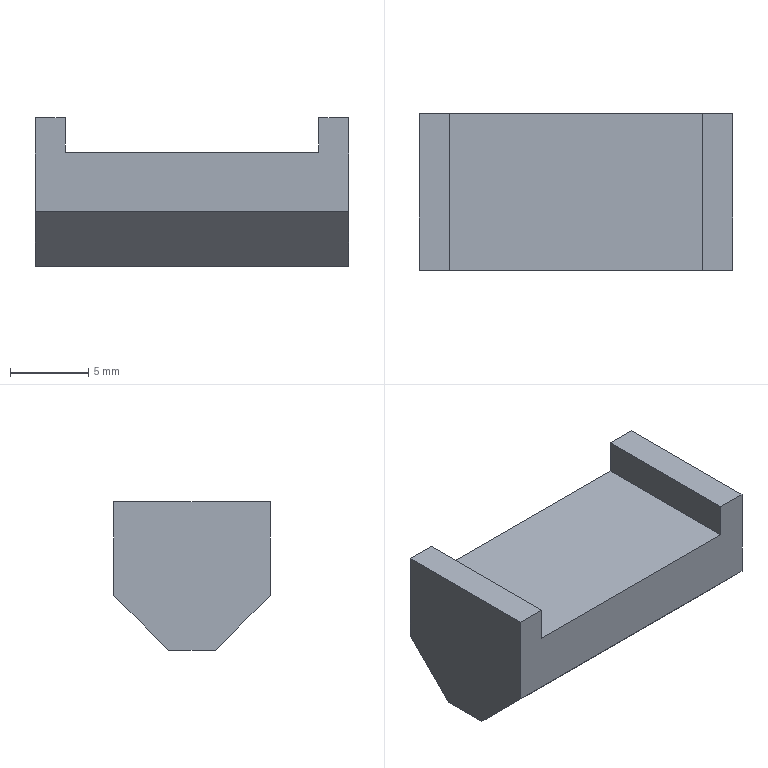Part | SolidWorks | features ICE 2, Extrusion 1, MirrorPattern 1 | 1 solid | 12 faces | box 20 x 10 x 9.5 mm | volume 1299 mm3 | plane 12
STEP:
#1=CARTESIAN_POINT('',(-10.,-1.5,0.));
#2=VERTEX_POINT('',#1);
#3=CARTESIAN_POINT('',(-10.,-5.,3.5));
#4=VERTEX_POINT('',#3);
#5=CARTESIAN_POINT('',(-10.,-5.,3.5));
#6=DIRECTION('',(0.,-0.7071,0.7071));
#7=VECTOR('',#6,1000.);
#8=LINE('',#5,#7);
#9=EDGE_CURVE('',#2,#4,#8,.T.);
#10=ORIENTED_EDGE('',*,*,#9,.T.);
#11=CARTESIAN_POINT('',(-10.,-5.,9.5));
#12=VERTEX_POINT('',#11);
#13=CARTESIAN_POINT('',(-10.,-5.,9.5));
#14=DIRECTION('',(0.,0.,-1.));
#15=VECTOR('',#14,1000.);
#16=LINE('',#13,#15);
#17=EDGE_CURVE('',#12,#4,#16,.T.);
#18=ORIENTED_EDGE('',*,*,#17,.F.);
#19=CARTESIAN_POINT('',(-10.,5.,9.5));
#20=VERTEX_POINT('',#19);
#21=CARTESIAN_POINT('',(-10.,5.,9.5));
#22=DIRECTION('',(0.,-1.,0.));
#23=VECTOR('',#22,1000.);
#24=LINE('',#21,#23);
#25=EDGE_CURVE('',#20,#12,#24,.T.);
#26=ORIENTED_EDGE('',*,*,#25,.F.);
#27=CARTESIAN_POINT('',(-10.,5.,3.5));
#28=VERTEX_POINT('',#27);
#29=CARTESIAN_POINT('',(-10.,5.,9.5));
#30=DIRECTION('',(0.,0.,-1.));
#31=VECTOR('',#30,1000.);
#32=LINE('',#29,#31);
#33=EDGE_CURVE('',#20,#28,#32,.T.);
#34=ORIENTED_EDGE('',*,*,#33,.T.);
#35=CARTESIAN_POINT('',(-10.,1.5,0.));
#36=VERTEX_POINT('',#35);
#37=CARTESIAN_POINT('',(-10.,5.,3.5));
#38=DIRECTION('',(0.,0.7071,0.7071));
#39=VECTOR('',#38,1000.);
#40=LINE('',#37,#39);
#41=EDGE_CURVE('',#36,#28,#40,.T.);
#42=ORIENTED_EDGE('',*,*,#41,.F.);
#43=CARTESIAN_POINT('',(-10.,5.,0.));
#44=DIRECTION('',(0.,-1.,0.));
#45=VECTOR('',#44,1000.);
#46=LINE('',#43,#45);
#47=EDGE_CURVE('',#36,#2,#46,.T.);
#48=ORIENTED_EDGE('',*,*,#47,.T.);
#49=EDGE_LOOP('',(#10,#18,#26,#34,#42,#48));
#50=FACE_OUTER_BOUND('',#49,.T.);
#51=CARTESIAN_POINT('',(-10.,5.,9.5));
#52=DIRECTION('',(1.,0.,0.));
#53=DIRECTION('',(0.,0.,-1.));
#54=AXIS2_PLACEMENT_3D('',#51,#52,#53);
#55=PLANE('',#54);
#56=ADVANCED_FACE('',(#50),#55,.F.);
#57=CARTESIAN_POINT('',(10.,-5.,3.5));
#58=VERTEX_POINT('',#57);
#59=CARTESIAN_POINT('',(10.,-5.,3.5));
#60=DIRECTION('',(-1.,0.,0.));
#61=VECTOR('',#60,1000.);
#62=LINE('',#59,#61);
#63=EDGE_CURVE('',#58,#4,#62,.T.);
#64=ORIENTED_EDGE('',*,*,#63,.F.);
#65=CARTESIAN_POINT('',(10.,-5.,9.5));
#66=VERTEX_POINT('',#65);
#67=CARTESIAN_POINT('',(10.,-5.,9.5));
#68=DIRECTION('',(0.,0.,-1.));
#69=VECTOR('',#68,1000.);
#70=LINE('',#67,#69);
#71=EDGE_CURVE('',#66,#58,#70,.T.);
#72=ORIENTED_EDGE('',*,*,#71,.F.);
#73=CARTESIAN_POINT('',(8.1,-5.,9.5));
#74=VERTEX_POINT('',#73);
#75=CARTESIAN_POINT('',(-10.,-5.,9.5));
#76=DIRECTION('',(1.,0.,0.));
#77=VECTOR('',#76,1000.);
#78=LINE('',#75,#77);
#79=EDGE_CURVE('',#74,#66,#78,.T.);
#80=ORIENTED_EDGE('',*,*,#79,.F.);
#81=CARTESIAN_POINT('',(8.1,-5.,7.3));
#82=VERTEX_POINT('',#81);
#83=CARTESIAN_POINT('',(8.1,-5.,9.5));
#84=DIRECTION('',(0.,0.,-1.));
#85=VECTOR('',#84,1000.);
#86=LINE('',#83,#85);
#87=EDGE_CURVE('',#74,#82,#86,.T.);
#88=ORIENTED_EDGE('',*,*,#87,.T.);
#89=CARTESIAN_POINT('',(-8.1,-5.,7.3));
#90=VERTEX_POINT('',#89);
#91=CARTESIAN_POINT('',(-10.,-5.,7.3));
#92=DIRECTION('',(1.,0.,0.));
#93=VECTOR('',#92,1000.);
#94=LINE('',#91,#93);
#95=EDGE_CURVE('',#90,#82,#94,.T.);
#96=ORIENTED_EDGE('',*,*,#95,.F.);
#97=CARTESIAN_POINT('',(-8.1,-5.,9.5));
#98=VERTEX_POINT('',#97);
#99=CARTESIAN_POINT('',(-8.1,-5.,9.5));
#100=DIRECTION('',(0.,0.,1.));
#101=VECTOR('',#100,1000.);
#102=LINE('',#99,#101);
#103=EDGE_CURVE('',#90,#98,#102,.T.);
#104=ORIENTED_EDGE('',*,*,#103,.T.);
#105=CARTESIAN_POINT('',(-10.,-5.,9.5));
#106=DIRECTION('',(1.,0.,0.));
#107=VECTOR('',#106,1000.);
#108=LINE('',#105,#107);
#109=EDGE_CURVE('',#12,#98,#108,.T.);
#110=ORIENTED_EDGE('',*,*,#109,.F.);
#111=ORIENTED_EDGE('',*,*,#17,.T.);
#112=EDGE_LOOP('',(#64,#72,#80,#88,#96,#104,#110,#111));
#113=FACE_OUTER_BOUND('',#112,.T.);
#114=CARTESIAN_POINT('',(-10.,-5.,9.5));
#115=DIRECTION('',(0.,1.,0.));
#116=DIRECTION('',(0.,0.,1.));
#117=AXIS2_PLACEMENT_3D('',#114,#115,#116);
#118=PLANE('',#117);
#119=ADVANCED_FACE('',(#113),#118,.F.);
#120=CARTESIAN_POINT('',(10.,-1.5,0.));
#121=VERTEX_POINT('',#120);
#122=CARTESIAN_POINT('',(10.,-5.,3.5));
#123=DIRECTION('',(0.,-0.7071,0.7071));
#124=VECTOR('',#123,1000.);
#125=LINE('',#122,#124);
#126=EDGE_CURVE('',#121,#58,#125,.T.);
#127=ORIENTED_EDGE('',*,*,#126,.F.);
#128=CARTESIAN_POINT('',(10.,1.5,0.));
#129=VERTEX_POINT('',#128);
#130=CARTESIAN_POINT('',(10.,5.,0.));
#131=DIRECTION('',(0.,1.,0.));
#132=VECTOR('',#131,1000.);
#133=LINE('',#130,#132);
#134=EDGE_CURVE('',#121,#129,#133,.T.);
#135=ORIENTED_EDGE('',*,*,#134,.T.);
#136=CARTESIAN_POINT('',(10.,5.,3.5));
#137=VERTEX_POINT('',#136);
#138=CARTESIAN_POINT('',(10.,5.,3.5));
#139=DIRECTION('',(0.,0.7071,0.7071));
#140=VECTOR('',#139,1000.);
#141=LINE('',#138,#140);
#142=EDGE_CURVE('',#129,#137,#141,.T.);
#143=ORIENTED_EDGE('',*,*,#142,.T.);
#144=CARTESIAN_POINT('',(10.,5.,9.5));
#145=VERTEX_POINT('',#144);
#146=CARTESIAN_POINT('',(10.,5.,9.5));
#147=DIRECTION('',(0.,0.,-1.));
#148=VECTOR('',#147,1000.);
#149=LINE('',#146,#148);
#150=EDGE_CURVE('',#145,#137,#149,.T.);
#151=ORIENTED_EDGE('',*,*,#150,.F.);
#152=CARTESIAN_POINT('',(10.,5.,9.5));
#153=DIRECTION('',(0.,1.,0.));
#154=VECTOR('',#153,1000.);
#155=LINE('',#152,#154);
#156=EDGE_CURVE('',#66,#145,#155,.T.);
#157=ORIENTED_EDGE('',*,*,#156,.F.);
#158=ORIENTED_EDGE('',*,*,#71,.T.);
#159=EDGE_LOOP('',(#127,#135,#143,#151,#157,#158));
#160=FACE_OUTER_BOUND('',#159,.T.);
#161=CARTESIAN_POINT('',(10.,5.,9.5));
#162=DIRECTION('',(-1.,0.,0.));
#163=DIRECTION('',(0.,0.,1.));
#164=AXIS2_PLACEMENT_3D('',#161,#162,#163);
#165=PLANE('',#164);
#166=ADVANCED_FACE('',(#160),#165,.F.);
#167=CARTESIAN_POINT('',(10.,-1.5,0.));
#168=DIRECTION('',(-1.,0.,0.));
#169=VECTOR('',#168,1000.);
#170=LINE('',#167,#169);
#171=EDGE_CURVE('',#121,#2,#170,.T.);
#172=ORIENTED_EDGE('',*,*,#171,.T.);
#173=ORIENTED_EDGE('',*,*,#47,.F.);
#174=CARTESIAN_POINT('',(10.,1.5,0.));
#175=DIRECTION('',(-1.,0.,0.));
#176=VECTOR('',#175,1000.);
#177=LINE('',#174,#176);
#178=EDGE_CURVE('',#129,#36,#177,.T.);
#179=ORIENTED_EDGE('',*,*,#178,.F.);
#180=ORIENTED_EDGE('',*,*,#134,.F.);
#181=EDGE_LOOP('',(#172,#173,#179,#180));
#182=FACE_OUTER_BOUND('',#181,.T.);
#183=CARTESIAN_POINT('',(0.,0.,0.));
#184=DIRECTION('',(0.,0.,1.));
#185=DIRECTION('',(1.,0.,0.));
#186=AXIS2_PLACEMENT_3D('',#183,#184,#185);
#187=PLANE('',#186);
#188=ADVANCED_FACE('',(#182),#187,.F.);
#189=CARTESIAN_POINT('',(-8.1,5.,9.5));
#190=VERTEX_POINT('',#189);
#191=CARTESIAN_POINT('',(-8.1,0.,9.5));
#192=DIRECTION('',(0.,-1.,0.));
#193=VECTOR('',#192,1000.);
#194=LINE('',#191,#193);
#195=EDGE_CURVE('',#190,#98,#194,.T.);
#196=ORIENTED_EDGE('',*,*,#195,.F.);
#197=CARTESIAN_POINT('',(-10.,5.,9.5));
#198=DIRECTION('',(-1.,0.,0.));
#199=VECTOR('',#198,1000.);
#200=LINE('',#197,#199);
#201=EDGE_CURVE('',#190,#20,#200,.T.);
#202=ORIENTED_EDGE('',*,*,#201,.T.);
#203=ORIENTED_EDGE('',*,*,#25,.T.);
#204=ORIENTED_EDGE('',*,*,#109,.T.);
#205=EDGE_LOOP('',(#196,#202,#203,#204));
#206=FACE_OUTER_BOUND('',#205,.T.);
#207=CARTESIAN_POINT('',(0.,0.,9.5));
#208=DIRECTION('',(0.,0.,1.));
#209=DIRECTION('',(1.,0.,0.));
#210=AXIS2_PLACEMENT_3D('',#207,#208,#209);
#211=PLANE('',#210);
#212=ADVANCED_FACE('',(#206),#211,.T.);
#213=ORIENTED_EDGE('',*,*,#150,.T.);
#214=CARTESIAN_POINT('',(10.,5.,3.5));
#215=DIRECTION('',(-1.,0.,0.));
#216=VECTOR('',#215,1000.);
#217=LINE('',#214,#216);
#218=EDGE_CURVE('',#137,#28,#217,.T.);
#219=ORIENTED_EDGE('',*,*,#218,.T.);
#220=ORIENTED_EDGE('',*,*,#33,.F.);
#221=ORIENTED_EDGE('',*,*,#201,.F.);
#222=CARTESIAN_POINT('',(-8.1,5.,7.3));
#223=VERTEX_POINT('',#222);
#224=CARTESIAN_POINT('',(-8.1,5.,9.5));
#225=DIRECTION('',(0.,0.,-1.));
#226=VECTOR('',#225,1000.);
#227=LINE('',#224,#226);
#228=EDGE_CURVE('',#190,#223,#227,.T.);
#229=ORIENTED_EDGE('',*,*,#228,.T.);
#230=CARTESIAN_POINT('',(8.1,5.,7.3));
#231=VERTEX_POINT('',#230);
#232=CARTESIAN_POINT('',(-10.,5.,7.3));
#233=DIRECTION('',(-1.,0.,0.));
#234=VECTOR('',#233,1000.);
#235=LINE('',#232,#234);
#236=EDGE_CURVE('',#231,#223,#235,.T.);
#237=ORIENTED_EDGE('',*,*,#236,.F.);
#238=CARTESIAN_POINT('',(8.1,5.,9.5));
#239=VERTEX_POINT('',#238);
#240=CARTESIAN_POINT('',(8.1,5.,9.5));
#241=DIRECTION('',(0.,0.,1.));
#242=VECTOR('',#241,1000.);
#243=LINE('',#240,#242);
#244=EDGE_CURVE('',#231,#239,#243,.T.);
#245=ORIENTED_EDGE('',*,*,#244,.T.);
#246=CARTESIAN_POINT('',(-10.,5.,9.5));
#247=DIRECTION('',(-1.,0.,0.));
#248=VECTOR('',#247,1000.);
#249=LINE('',#246,#248);
#250=EDGE_CURVE('',#145,#239,#249,.T.);
#251=ORIENTED_EDGE('',*,*,#250,.F.);
#252=EDGE_LOOP('',(#213,#219,#220,#221,#229,#237,#245,#251));
#253=FACE_OUTER_BOUND('',#252,.T.);
#254=CARTESIAN_POINT('',(-10.,5.,9.5));
#255=DIRECTION('',(0.,-1.,0.));
#256=DIRECTION('',(0.,0.,-1.));
#257=AXIS2_PLACEMENT_3D('',#254,#255,#256);
#258=PLANE('',#257);
#259=ADVANCED_FACE('',(#253),#258,.F.);
#260=CARTESIAN_POINT('',(8.1,0.,9.5));
#261=DIRECTION('',(0.,1.,0.));
#262=VECTOR('',#261,1000.);
#263=LINE('',#260,#262);
#264=EDGE_CURVE('',#74,#239,#263,.T.);
#265=ORIENTED_EDGE('',*,*,#264,.F.);
#266=ORIENTED_EDGE('',*,*,#79,.T.);
#267=ORIENTED_EDGE('',*,*,#156,.T.);
#268=ORIENTED_EDGE('',*,*,#250,.T.);
#269=EDGE_LOOP('',(#265,#266,#267,#268));
#270=FACE_OUTER_BOUND('',#269,.T.);
#271=CARTESIAN_POINT('',(0.,0.,9.5));
#272=DIRECTION('',(0.,0.,1.));
#273=DIRECTION('',(1.,0.,0.));
#274=AXIS2_PLACEMENT_3D('',#271,#272,#273);
#275=PLANE('',#274);
#276=ADVANCED_FACE('',(#270),#275,.T.);
#277=ORIENTED_EDGE('',*,*,#95,.T.);
#278=CARTESIAN_POINT('',(8.1,14.948,7.3));
#279=DIRECTION('',(0.,1.,0.));
#280=VECTOR('',#279,1000.);
#281=LINE('',#278,#280);
#282=EDGE_CURVE('',#82,#231,#281,.T.);
#283=ORIENTED_EDGE('',*,*,#282,.T.);
#284=ORIENTED_EDGE('',*,*,#236,.T.);
#285=CARTESIAN_POINT('',(-8.1,14.948,7.3));
#286=DIRECTION('',(0.,-1.,0.));
#287=VECTOR('',#286,1000.);
#288=LINE('',#285,#287);
#289=EDGE_CURVE('',#223,#90,#288,.T.);
#290=ORIENTED_EDGE('',*,*,#289,.T.);
#291=EDGE_LOOP('',(#277,#283,#284,#290));
#292=FACE_OUTER_BOUND('',#291,.T.);
#293=CARTESIAN_POINT('',(0.,0.,7.3));
#294=DIRECTION('',(0.,0.,1.));
#295=DIRECTION('',(1.,0.,0.));
#296=AXIS2_PLACEMENT_3D('',#293,#294,#295);
#297=PLANE('',#296);
#298=ADVANCED_FACE('',(#292),#297,.T.);
#299=ORIENTED_EDGE('',*,*,#289,.F.);
#300=ORIENTED_EDGE('',*,*,#228,.F.);
#301=ORIENTED_EDGE('',*,*,#195,.T.);
#302=ORIENTED_EDGE('',*,*,#103,.F.);
#303=EDGE_LOOP('',(#299,#300,#301,#302));
#304=FACE_OUTER_BOUND('',#303,.T.);
#305=CARTESIAN_POINT('',(-8.1,14.948,7.3));
#306=DIRECTION('',(-1.,0.,0.));
#307=DIRECTION('',(0.,0.,1.));
#308=AXIS2_PLACEMENT_3D('',#305,#306,#307);
#309=PLANE('',#308);
#310=ADVANCED_FACE('',(#304),#309,.F.);
#311=ORIENTED_EDGE('',*,*,#264,.T.);
#312=ORIENTED_EDGE('',*,*,#244,.F.);
#313=ORIENTED_EDGE('',*,*,#282,.F.);
#314=ORIENTED_EDGE('',*,*,#87,.F.);
#315=EDGE_LOOP('',(#311,#312,#313,#314));
#316=FACE_OUTER_BOUND('',#315,.T.);
#317=CARTESIAN_POINT('',(8.1,14.948,7.3));
#318=DIRECTION('',(1.,0.,0.));
#319=DIRECTION('',(0.,0.,-1.));
#320=AXIS2_PLACEMENT_3D('',#317,#318,#319);
#321=PLANE('',#320);
#322=ADVANCED_FACE('',(#316),#321,.F.);
#323=ORIENTED_EDGE('',*,*,#41,.T.);
#324=ORIENTED_EDGE('',*,*,#218,.F.);
#325=ORIENTED_EDGE('',*,*,#142,.F.);
#326=ORIENTED_EDGE('',*,*,#178,.T.);
#327=EDGE_LOOP('',(#323,#324,#325,#326));
#328=FACE_OUTER_BOUND('',#327,.T.);
#329=CARTESIAN_POINT('',(10.,5.,3.5));
#330=DIRECTION('',(0.,-0.7071,0.7071));
#331=DIRECTION('',(0.,-0.7071,-0.7071));
#332=AXIS2_PLACEMENT_3D('',#329,#330,#331);
#333=PLANE('',#332);
#334=ADVANCED_FACE('',(#328),#333,.F.);
#335=ORIENTED_EDGE('',*,*,#9,.F.);
#336=ORIENTED_EDGE('',*,*,#171,.F.);
#337=ORIENTED_EDGE('',*,*,#126,.T.);
#338=ORIENTED_EDGE('',*,*,#63,.T.);
#339=EDGE_LOOP('',(#335,#336,#337,#338));
#340=FACE_OUTER_BOUND('',#339,.T.);
#341=CARTESIAN_POINT('',(10.,-5.,3.5));
#342=DIRECTION('',(0.,-0.7071,-0.7071));
#343=DIRECTION('',(0.,0.7071,-0.7071));
#344=AXIS2_PLACEMENT_3D('',#341,#342,#343);
#345=PLANE('',#344);
#346=ADVANCED_FACE('',(#340),#345,.T.);
#347=CLOSED_SHELL('',(#56,#119,#166,#188,#212,#259,#276,#298,#310,#322,#334,#346));
#348=MANIFOLD_SOLID_BREP('',#347);
#349=CARTESIAN_POINT('',(0.,0.,0.));
#350=DIRECTION('',(0.,0.,1.));
#351=DIRECTION('',(1.,0.,0.));
#352=AXIS2_PLACEMENT_3D('',#349,#350,#351);
#353=(LENGTH_UNIT()NAMED_UNIT(*)SI_UNIT(.MILLI.,.METRE.));
#354=UNCERTAINTY_MEASURE_WITH_UNIT(LENGTH_MEASURE(0.00001),#353,'','');
#355=(NAMED_UNIT(*)PLANE_ANGLE_UNIT()SI_UNIT($,.RADIAN.));
#356=(NAMED_UNIT(*)SI_UNIT($,.STERADIAN.)SOLID_ANGLE_UNIT());
#357=(GEOMETRIC_REPRESENTATION_CONTEXT(3)GLOBAL_UNCERTAINTY_ASSIGNED_CONTEXT((#354))GLOBAL_UNIT_ASSIGNED_CONTEXT((#353,#355,#356))REPRESENTATION_CONTEXT('',''));
#358=ADVANCED_BREP_SHAPE_REPRESENTATION('',(#348,#352),#357);